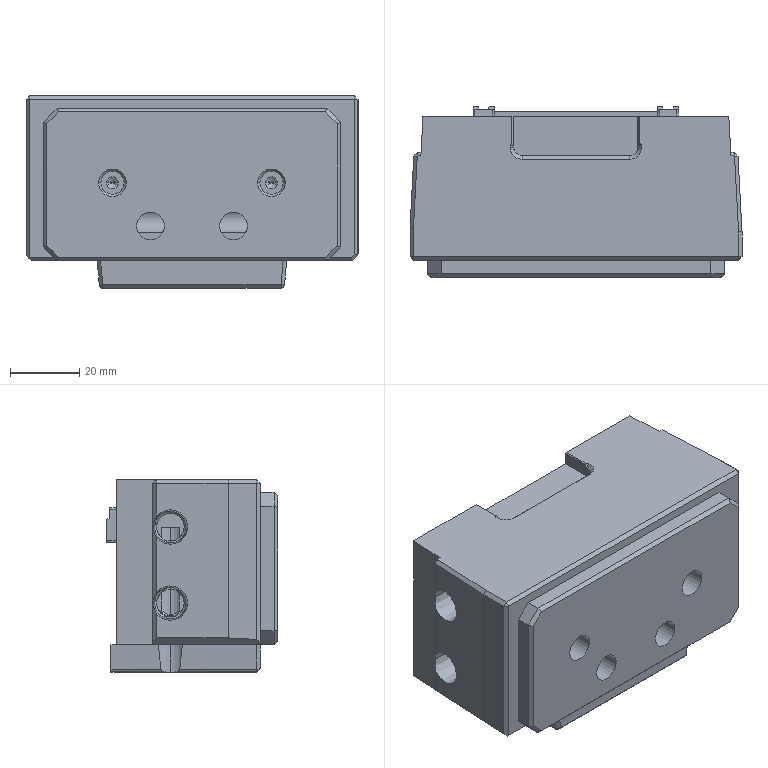Part | Creo | 1 solid | 218 faces | box 96 x 49.465 x 55.677 mm | volume 205257 mm3 | plane 123 | cylinder 53 | cone 26 | spline 11 | torus 5 | commonest cylinder face diameters 8 x22 7.5 x9 1.118 x8 2.01 x6 10 x4 5 x2